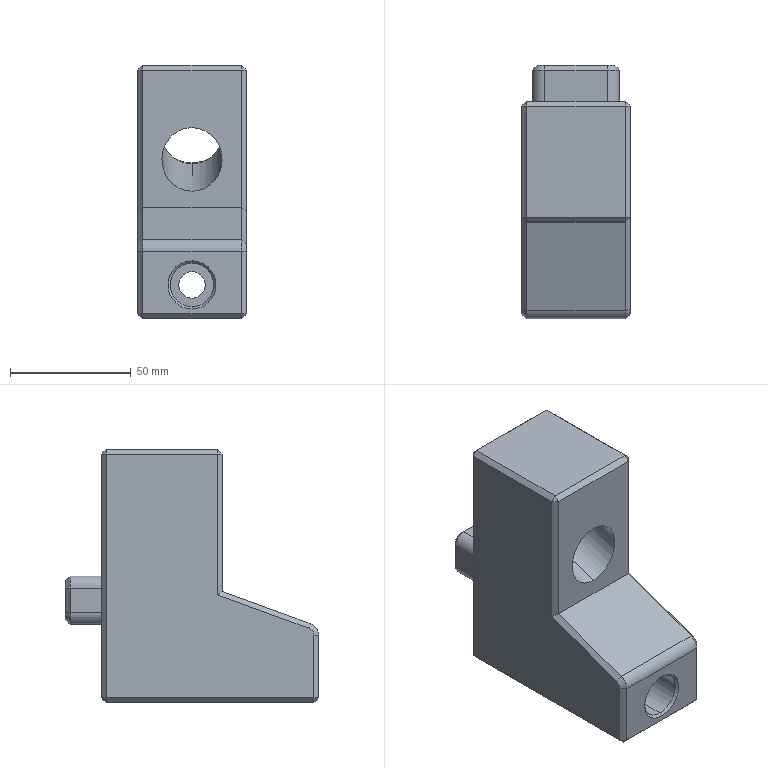Part | STEP file | Cunha 2 - Torre - 1 cav | 1 solid | 68 faces | box 45 x 105 x 105 mm | volume 266271 mm3 | plane 43 | cylinder 13 | cone 10 | spline 2 | commonest cylinder face diameters 10 x5 11 x2 18 x2 25 x2 33 x2